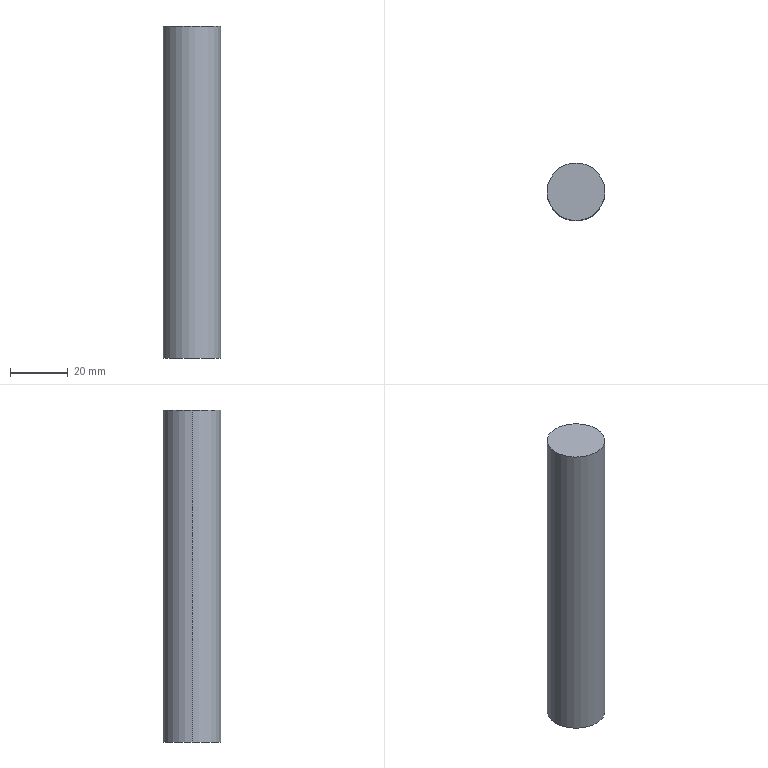Part | STEP file | 1 solid | 4 faces | box 20 x 20 x 115 mm | volume 36128 mm3 | cylinder 2 | plane 2 | commonest cylinder face diameters 20 x2
STEP:
#1=CARTESIAN_POINT('',(0.,0.,0.));
#2=DIRECTION('',(0.,0.,1.));
#3=DIRECTION('',(1.,0.,0.));
#4=AXIS2_PLACEMENT_3D('',#1,#2,#3);
#5=CARTESIAN_POINT('',(10.,1.493,-5.));
#6=VERTEX_POINT('',#5);
#7=CARTESIAN_POINT('',(-10.,1.493,-5.));
#8=VERTEX_POINT('',#7);
#9=CARTESIAN_POINT('',(0.,1.493,-5.));
#10=DIRECTION('',(0.,0.,1.));
#11=DIRECTION('',(1.,0.,0.));
#12=AXIS2_PLACEMENT_3D('',#9,#10,#11);
#13=CIRCLE('',#12,10.);
#14=CARTESIAN_POINT('',(0.,1.493,0.));
#15=DIRECTION('',(0.,0.,1.));
#16=DIRECTION('',(1.,0.,0.));
#17=AXIS2_PLACEMENT_3D('',#14,#15,#16);
#18=CYLINDRICAL_SURFACE('',#17,10.);
#19=CARTESIAN_POINT('',(0.,-5.));
#20=DIRECTION('',(1.,0.));
#21=VECTOR('',#20,1.);
#22=LINE('',#19,#21);
#23=(GEOMETRIC_REPRESENTATION_CONTEXT(2)PARAMETRIC_REPRESENTATION_CONTEXT()REPRESENTATION_CONTEXT('',''));
#24=DEFINITIONAL_REPRESENTATION('',(#22),#23);
#25=PCURVE('',#18,#24);
#26=CARTESIAN_POINT('',(0.,1.493,-5.));
#27=DIRECTION('',(0.,0.,1.));
#28=DIRECTION('',(1.,0.,0.));
#29=AXIS2_PLACEMENT_3D('',#26,#27,#28);
#30=PLANE('',#29);
#31=CARTESIAN_POINT('',(0.,0.));
#32=DIRECTION('',(1.,0.));
#33=AXIS2_PLACEMENT_2D('',#31,#32);
#34=CIRCLE('',#33,10.);
#35=(GEOMETRIC_REPRESENTATION_CONTEXT(2)PARAMETRIC_REPRESENTATION_CONTEXT()REPRESENTATION_CONTEXT('',''));
#36=DEFINITIONAL_REPRESENTATION('',(#34),#35);
#37=PCURVE('',#30,#36);
#38=SURFACE_CURVE('',#13,(#25,#37),.PCURVE_S1.);
#39=EDGE_CURVE('',#6,#8,#38,.T.);
#40=ORIENTED_EDGE('',*,*,#39,.T.);
#41=CARTESIAN_POINT('',(-10.,1.493,110.));
#42=VERTEX_POINT('',#41);
#43=CARTESIAN_POINT('',(-10.,1.493,0.));
#44=DIRECTION('',(0.,0.,1.));
#45=VECTOR('',#44,1.);
#46=LINE('',#43,#45);
#47=CARTESIAN_POINT('',(3.142,0.));
#48=DIRECTION('',(0.,1.));
#49=VECTOR('',#48,1.);
#50=LINE('',#47,#49);
#51=(GEOMETRIC_REPRESENTATION_CONTEXT(2)PARAMETRIC_REPRESENTATION_CONTEXT()REPRESENTATION_CONTEXT('',''));
#52=DEFINITIONAL_REPRESENTATION('',(#50),#51);
#53=PCURVE('',#18,#52);
#54=CARTESIAN_POINT('',(0.,1.493,0.));
#55=DIRECTION('',(0.,0.,1.));
#56=DIRECTION('',(1.,0.,0.));
#57=AXIS2_PLACEMENT_3D('',#54,#55,#56);
#58=CYLINDRICAL_SURFACE('',#57,10.);
#59=CARTESIAN_POINT('',(3.142,0.));
#60=DIRECTION('',(0.,1.));
#61=VECTOR('',#60,1.);
#62=LINE('',#59,#61);
#63=(GEOMETRIC_REPRESENTATION_CONTEXT(2)PARAMETRIC_REPRESENTATION_CONTEXT()REPRESENTATION_CONTEXT('',''));
#64=DEFINITIONAL_REPRESENTATION('',(#62),#63);
#65=PCURVE('',#58,#64);
#66=SURFACE_CURVE('',#46,(#53,#65),.PCURVE_S1.);
#67=EDGE_CURVE('',#8,#42,#66,.T.);
#68=ORIENTED_EDGE('',*,*,#67,.T.);
#69=CARTESIAN_POINT('',(10.,1.493,110.));
#70=VERTEX_POINT('',#69);
#71=CARTESIAN_POINT('',(0.,1.493,110.));
#72=DIRECTION('',(0.,0.,-1.));
#73=DIRECTION('',(1.,0.,0.));
#74=AXIS2_PLACEMENT_3D('',#71,#72,#73);
#75=CIRCLE('',#74,10.);
#76=CARTESIAN_POINT('',(6.283,110.));
#77=DIRECTION('',(-1.,0.));
#78=VECTOR('',#77,1.);
#79=LINE('',#76,#78);
#80=(GEOMETRIC_REPRESENTATION_CONTEXT(2)PARAMETRIC_REPRESENTATION_CONTEXT()REPRESENTATION_CONTEXT('',''));
#81=DEFINITIONAL_REPRESENTATION('',(#79),#80);
#82=PCURVE('',#18,#81);
#83=CARTESIAN_POINT('',(0.,1.493,110.));
#84=DIRECTION('',(0.,0.,1.));
#85=DIRECTION('',(1.,0.,0.));
#86=AXIS2_PLACEMENT_3D('',#83,#84,#85);
#87=PLANE('',#86);
#88=CARTESIAN_POINT('',(10.,0.));
#89=CARTESIAN_POINT('',(10.,-17.321));
#90=CARTESIAN_POINT('',(-5.,-8.66));
#91=CARTESIAN_POINT('',(-20.,0.));
#92=CARTESIAN_POINT('',(-5.,8.66));
#93=CARTESIAN_POINT('',(10.,17.321));
#94=CARTESIAN_POINT('',(10.,0.));
#95=(BOUNDED_CURVE()B_SPLINE_CURVE(2,(#88,#89,#90,#91,#92,#93,#94),.UNSPECIFIED.,.T.,.F.)B_SPLINE_CURVE_WITH_KNOTS((1,2,2,2,2,1),(-2.094,0.,2.094,4.189,6.283,8.378),.UNSPECIFIED.)CURVE()GEOMETRIC_REPRESENTATION_ITEM()RATIONAL_B_SPLINE_CURVE((1.,0.5,1.,0.5,1.,0.5,1.))REPRESENTATION_ITEM(''));
#96=(GEOMETRIC_REPRESENTATION_CONTEXT(2)PARAMETRIC_REPRESENTATION_CONTEXT()REPRESENTATION_CONTEXT('',''));
#97=DEFINITIONAL_REPRESENTATION('',(#95),#96);
#98=PCURVE('',#87,#97);
#99=SURFACE_CURVE('',#75,(#82,#98),.PCURVE_S1.);
#100=EDGE_CURVE('',#42,#70,#99,.T.);
#101=ORIENTED_EDGE('',*,*,#100,.T.);
#102=CARTESIAN_POINT('',(10.,1.493,0.));
#103=DIRECTION('',(0.,0.,1.));
#104=VECTOR('',#103,1.);
#105=LINE('',#102,#104);
#106=CARTESIAN_POINT('',(0.,0.));
#107=DIRECTION('',(0.,1.));
#108=VECTOR('',#107,1.);
#109=LINE('',#106,#108);
#110=(GEOMETRIC_REPRESENTATION_CONTEXT(2)PARAMETRIC_REPRESENTATION_CONTEXT()REPRESENTATION_CONTEXT('',''));
#111=DEFINITIONAL_REPRESENTATION('',(#109),#110);
#112=PCURVE('',#18,#111);
#113=CARTESIAN_POINT('',(6.283,0.));
#114=DIRECTION('',(0.,1.));
#115=VECTOR('',#114,1.);
#116=LINE('',#113,#115);
#117=(GEOMETRIC_REPRESENTATION_CONTEXT(2)PARAMETRIC_REPRESENTATION_CONTEXT()REPRESENTATION_CONTEXT('',''));
#118=DEFINITIONAL_REPRESENTATION('',(#116),#117);
#119=PCURVE('',#58,#118);
#120=SURFACE_CURVE('',#105,(#112,#119),.PCURVE_S1.);
#121=EDGE_CURVE('',#6,#70,#120,.T.);
#122=ORIENTED_EDGE('',*,*,#121,.F.);
#123=EDGE_LOOP('',(#40,#68,#101,#122));
#124=FACE_BOUND('',#123,.T.);
#125=ADVANCED_FACE('',(#124),#18,.T.);
#126=ORIENTED_EDGE('',*,*,#67,.F.);
#127=CARTESIAN_POINT('',(0.,1.493,-5.));
#128=DIRECTION('',(0.,0.,1.));
#129=DIRECTION('',(1.,0.,0.));
#130=AXIS2_PLACEMENT_3D('',#127,#128,#129);
#131=CIRCLE('',#130,10.);
#132=CARTESIAN_POINT('',(0.,-5.));
#133=DIRECTION('',(1.,0.));
#134=VECTOR('',#133,1.);
#135=LINE('',#132,#134);
#136=(GEOMETRIC_REPRESENTATION_CONTEXT(2)PARAMETRIC_REPRESENTATION_CONTEXT()REPRESENTATION_CONTEXT('',''));
#137=DEFINITIONAL_REPRESENTATION('',(#135),#136);
#138=PCURVE('',#58,#137);
#139=CARTESIAN_POINT('',(0.,0.));
#140=DIRECTION('',(1.,0.));
#141=AXIS2_PLACEMENT_2D('',#139,#140);
#142=CIRCLE('',#141,10.);
#143=(GEOMETRIC_REPRESENTATION_CONTEXT(2)PARAMETRIC_REPRESENTATION_CONTEXT()REPRESENTATION_CONTEXT('',''));
#144=DEFINITIONAL_REPRESENTATION('',(#142),#143);
#145=PCURVE('',#30,#144);
#146=SURFACE_CURVE('',#131,(#138,#145),.PCURVE_S1.);
#147=EDGE_CURVE('',#8,#6,#146,.T.);
#148=ORIENTED_EDGE('',*,*,#147,.T.);
#149=ORIENTED_EDGE('',*,*,#121,.T.);
#150=CARTESIAN_POINT('',(0.,1.493,110.));
#151=DIRECTION('',(0.,0.,-1.));
#152=DIRECTION('',(1.,0.,0.));
#153=AXIS2_PLACEMENT_3D('',#150,#151,#152);
#154=CIRCLE('',#153,10.);
#155=CARTESIAN_POINT('',(6.283,110.));
#156=DIRECTION('',(-1.,0.));
#157=VECTOR('',#156,1.);
#158=LINE('',#155,#157);
#159=(GEOMETRIC_REPRESENTATION_CONTEXT(2)PARAMETRIC_REPRESENTATION_CONTEXT()REPRESENTATION_CONTEXT('',''));
#160=DEFINITIONAL_REPRESENTATION('',(#158),#159);
#161=PCURVE('',#58,#160);
#162=CARTESIAN_POINT('',(10.,0.));
#163=CARTESIAN_POINT('',(10.,-17.321));
#164=CARTESIAN_POINT('',(-5.,-8.66));
#165=CARTESIAN_POINT('',(-20.,0.));
#166=CARTESIAN_POINT('',(-5.,8.66));
#167=CARTESIAN_POINT('',(10.,17.321));
#168=CARTESIAN_POINT('',(10.,0.));
#169=(BOUNDED_CURVE()B_SPLINE_CURVE(2,(#162,#163,#164,#165,#166,#167,#168),.UNSPECIFIED.,.T.,.F.)B_SPLINE_CURVE_WITH_KNOTS((1,2,2,2,2,1),(-2.094,0.,2.094,4.189,6.283,8.378),.UNSPECIFIED.)CURVE()GEOMETRIC_REPRESENTATION_ITEM()RATIONAL_B_SPLINE_CURVE((1.,0.5,1.,0.5,1.,0.5,1.))REPRESENTATION_ITEM(''));
#170=(GEOMETRIC_REPRESENTATION_CONTEXT(2)PARAMETRIC_REPRESENTATION_CONTEXT()REPRESENTATION_CONTEXT('',''));
#171=DEFINITIONAL_REPRESENTATION('',(#169),#170);
#172=PCURVE('',#87,#171);
#173=SURFACE_CURVE('',#154,(#161,#172),.PCURVE_S1.);
#174=EDGE_CURVE('',#70,#42,#173,.T.);
#175=ORIENTED_EDGE('',*,*,#174,.T.);
#176=EDGE_LOOP('',(#126,#148,#149,#175));
#177=FACE_BOUND('',#176,.T.);
#178=ADVANCED_FACE('',(#177),#58,.T.);
#179=ORIENTED_EDGE('',*,*,#174,.F.);
#180=ORIENTED_EDGE('',*,*,#100,.F.);
#181=EDGE_LOOP('',(#179,#180));
#182=FACE_BOUND('',#181,.T.);
#183=ADVANCED_FACE('',(#182),#87,.T.);
#184=ORIENTED_EDGE('',*,*,#39,.F.);
#185=ORIENTED_EDGE('',*,*,#147,.F.);
#186=EDGE_LOOP('',(#184,#185));
#187=FACE_BOUND('',#186,.T.);
#188=ADVANCED_FACE('',(#187),#30,.F.);
#189=CLOSED_SHELL('',(#125,#178,#183,#188));
#190=MANIFOLD_SOLID_BREP('',#189);
#191=(LENGTH_UNIT()NAMED_UNIT(*)SI_UNIT(.MILLI.,.METRE.));
#192=UNCERTAINTY_MEASURE_WITH_UNIT(LENGTH_MEASURE(0.0000001),#191,'','');
#193=(NAMED_UNIT(*)PLANE_ANGLE_UNIT()SI_UNIT($,.RADIAN.));
#194=(NAMED_UNIT(*)SI_UNIT($,.STERADIAN.)SOLID_ANGLE_UNIT());
#195=(GEOMETRIC_REPRESENTATION_CONTEXT(3)GLOBAL_UNCERTAINTY_ASSIGNED_CONTEXT((#192))GLOBAL_UNIT_ASSIGNED_CONTEXT((#191,#193,#194))REPRESENTATION_CONTEXT('',''));
#196=ADVANCED_BREP_SHAPE_REPRESENTATION('',(#4,#190),#195);